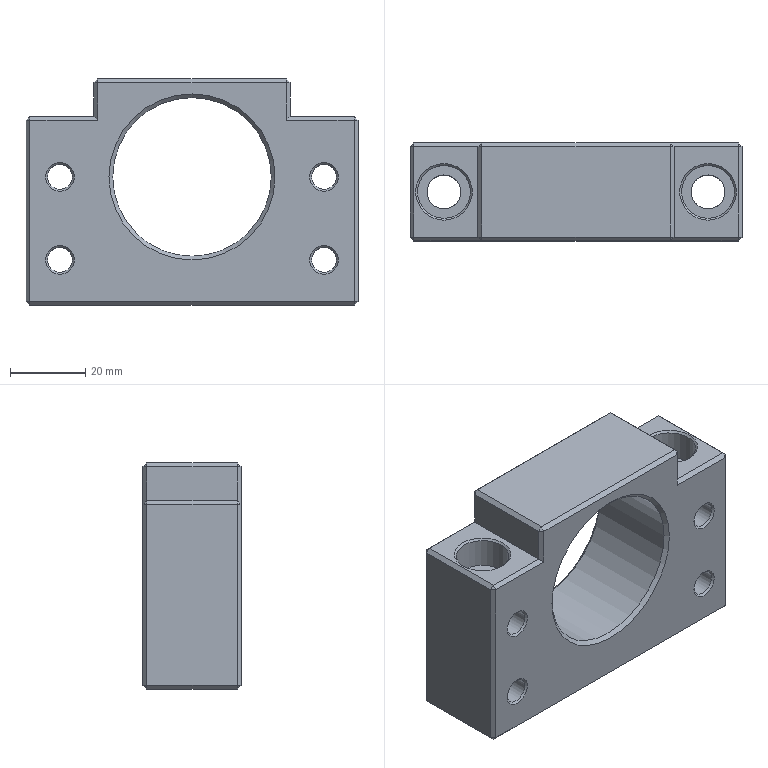Part | STEP file | BF-20_id1338_x_t | 1 solid | 71 faces | box 88 x 26 x 60 mm | volume 81051 mm3 | plane 46 | cylinder 13 | cone 12 | commonest cylinder face diameters 6.6 x8 9 x2 14 x2 42 x1